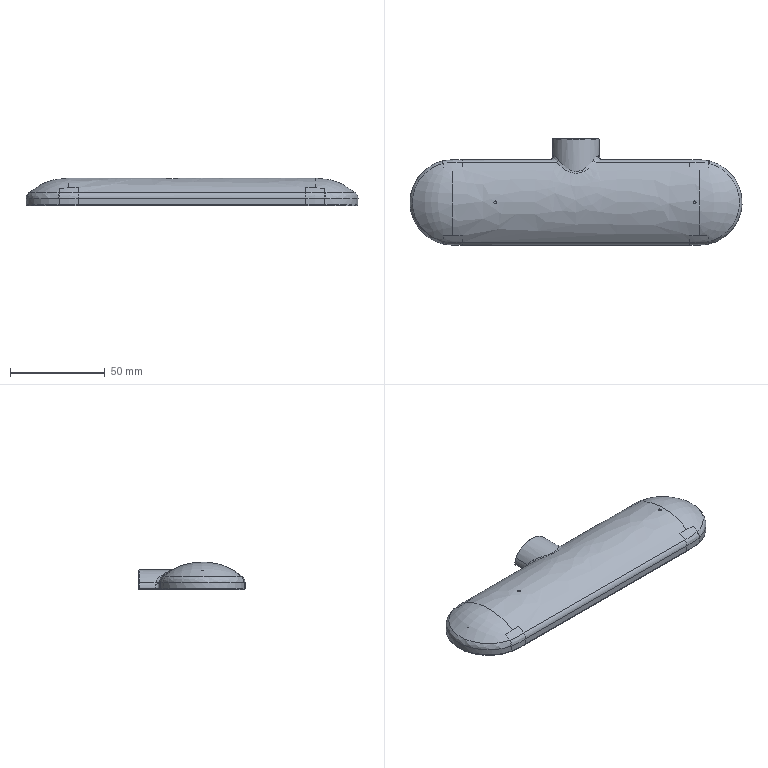Part | NX | features SKETCH 13, EXTRUDE 10, HOLE PACKAGE 7, SIMPLE HOLE 7, BLEND 5, DATUM_PLANE 3, EXTRACT_BODY 3, SEW 3, THRU_CURVE_MESH 3, BRIDGE_CURVE 2, Container 2, DATUM_CSYS 2, Geometry Instance 2, THRU_CURVE 2, CHAMFER 1, CPROJ 1, DRAFT 1, EXTRACT_FACE 1, SCALE 1, SWP104 1, THICKEN_SHEET 1, TRIM BODY 1, TRIM_AND_EXTEND 1, UNITE 1 | 1 solid | 151 faces | box 175 x 56.021 x 14.648 mm | volume 11136 mm3 | spline 70 | plane 37 | cylinder 32 | torus 7 | cone 5 | commonest cylinder face diameters 1.5 x7 5 x5 6 x3 8 x3 11.25 x2 13.25 x2